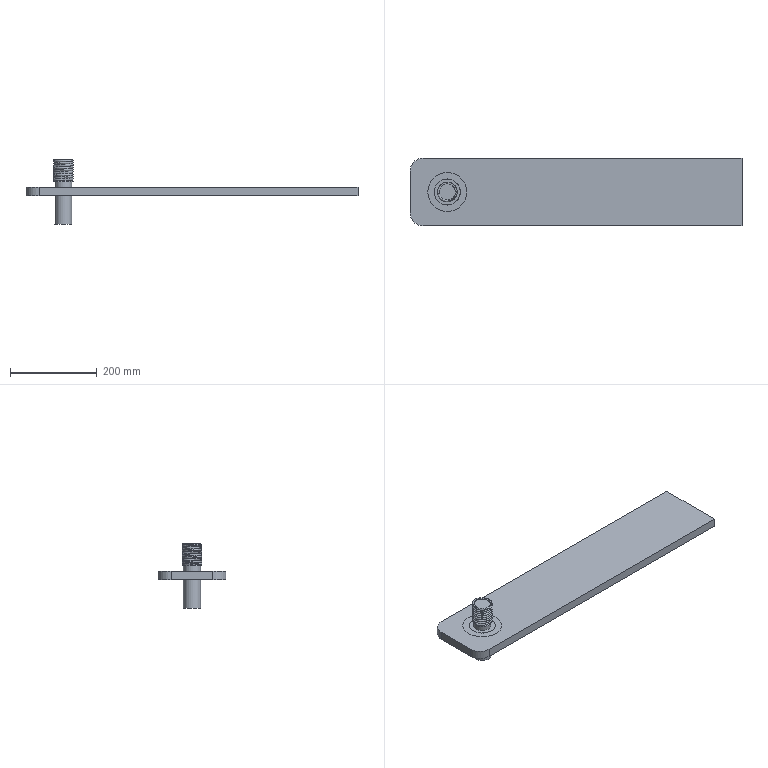Part | NX | features BREP 5 | 5 solids | 29 faces | box 765 x 156 x 148 mm | volume 2551294 mm3 | plane 16 | cylinder 8 | spline 5 | commonest cylinder face diameters 60 x4 40 x2 90 x2